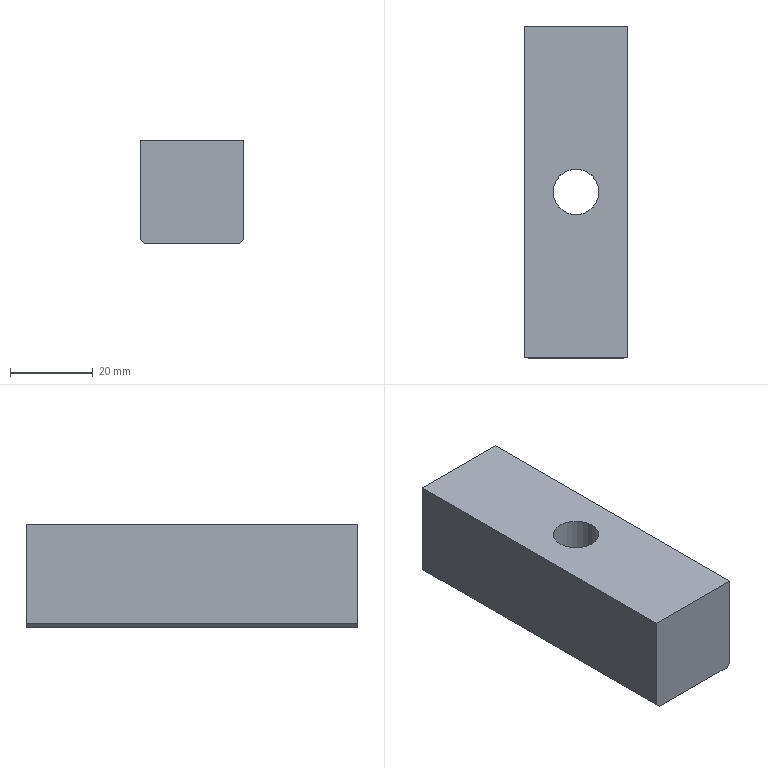Part | NX | features solid 2 | 1 solid | 11 faces | box 25 x 80 x 25 mm | volume 45631 mm3 | plane 9 | cylinder 2 | commonest cylinder face diameters 11 x1 18 x1
STEP:
#1=CARTESIAN_POINT('',(-5.5,1000.,-40.));
#2=VERTEX_POINT('',#1);
#3=CARTESIAN_POINT('',(0.,1000.,-40.));
#4=DIRECTION('',(0.,0.,-1.));
#5=DIRECTION('',(-1.,0.,0.));
#6=AXIS2_PLACEMENT_3D('',#3,#4,#5);
#7=CIRCLE('',#6,5.5);
#8=EDGE_CURVE('',#2,#2,#7,.T.);
#9=ORIENTED_EDGE('',*,*,#8,.T.);
#10=EDGE_LOOP('',(#9));
#11=FACE_BOUND('',#10,.T.);
#12=CARTESIAN_POINT('',(12.5,960.,-40.));
#13=VERTEX_POINT('',#12);
#14=CARTESIAN_POINT('',(-12.5,960.,-40.));
#15=VERTEX_POINT('',#14);
#16=CARTESIAN_POINT('',(0.,960.,-40.));
#17=DIRECTION('',(-1.,0.,0.));
#18=VECTOR('',#17,1000.);
#19=LINE('',#16,#18);
#20=EDGE_CURVE('',#13,#15,#19,.T.);
#21=ORIENTED_EDGE('',*,*,#20,.F.);
#22=CARTESIAN_POINT('',(12.5,1040.,-40.));
#23=VERTEX_POINT('',#22);
#24=CARTESIAN_POINT('',(12.5,1000.,-40.));
#25=DIRECTION('',(0.,-1.,0.));
#26=VECTOR('',#25,1000.);
#27=LINE('',#24,#26);
#28=EDGE_CURVE('',#23,#13,#27,.T.);
#29=ORIENTED_EDGE('',*,*,#28,.F.);
#30=CARTESIAN_POINT('',(-12.5,1040.,-40.));
#31=VERTEX_POINT('',#30);
#32=CARTESIAN_POINT('',(0.,1040.,-40.));
#33=DIRECTION('',(1.,0.,0.));
#34=VECTOR('',#33,1000.);
#35=LINE('',#32,#34);
#36=EDGE_CURVE('',#31,#23,#35,.T.);
#37=ORIENTED_EDGE('',*,*,#36,.F.);
#38=CARTESIAN_POINT('',(-12.5,1000.,-40.));
#39=DIRECTION('',(0.,1.,0.));
#40=VECTOR('',#39,1000.);
#41=LINE('',#38,#40);
#42=EDGE_CURVE('',#15,#31,#41,.T.);
#43=ORIENTED_EDGE('',*,*,#42,.F.);
#44=EDGE_LOOP('',(#21,#29,#37,#43));
#45=FACE_BOUND('',#44,.T.);
#46=CARTESIAN_POINT('',(0.,1000.,-40.));
#47=DIRECTION('',(0.,0.,1.));
#48=DIRECTION('',(1.,0.,0.));
#49=AXIS2_PLACEMENT_3D('',#46,#47,#48);
#50=PLANE('',#49);
#51=ADVANCED_FACE('',(#11,#45),#50,.T.);
#52=CARTESIAN_POINT('',(-11.5,960.,-65.));
#53=VERTEX_POINT('',#52);
#54=CARTESIAN_POINT('',(11.5,960.,-65.));
#55=VERTEX_POINT('',#54);
#56=CARTESIAN_POINT('',(0.,960.,-65.));
#57=DIRECTION('',(1.,0.,0.));
#58=VECTOR('',#57,1000.);
#59=LINE('',#56,#58);
#60=EDGE_CURVE('',#53,#55,#59,.T.);
#61=ORIENTED_EDGE('',*,*,#60,.T.);
#62=CARTESIAN_POINT('',(12.5,960.,-64.));
#63=VERTEX_POINT('',#62);
#64=CARTESIAN_POINT('',(5.75,960.,-70.75));
#65=DIRECTION('',(-0.7071,0.,-0.7071));
#66=VECTOR('',#65,1000.);
#67=LINE('',#64,#66);
#68=EDGE_CURVE('',#55,#63,#67,.F.);
#69=ORIENTED_EDGE('',*,*,#68,.T.);
#70=CARTESIAN_POINT('',(12.5,960.,-65.));
#71=DIRECTION('',(0.,0.,1.));
#72=VECTOR('',#71,1000.);
#73=LINE('',#70,#72);
#74=EDGE_CURVE('',#63,#13,#73,.T.);
#75=ORIENTED_EDGE('',*,*,#74,.T.);
#76=ORIENTED_EDGE('',*,*,#20,.T.);
#77=CARTESIAN_POINT('',(-12.5,960.,-64.));
#78=VERTEX_POINT('',#77);
#79=CARTESIAN_POINT('',(-12.5,960.,-65.));
#80=DIRECTION('',(0.,0.,1.));
#81=VECTOR('',#80,1000.);
#82=LINE('',#79,#81);
#83=EDGE_CURVE('',#78,#15,#82,.T.);
#84=ORIENTED_EDGE('',*,*,#83,.F.);
#85=CARTESIAN_POINT('',(-5.75,960.,-70.75));
#86=DIRECTION('',(-0.7071,0.,0.7071));
#87=VECTOR('',#86,1000.);
#88=LINE('',#85,#87);
#89=EDGE_CURVE('',#78,#53,#88,.F.);
#90=ORIENTED_EDGE('',*,*,#89,.T.);
#91=EDGE_LOOP('',(#61,#69,#75,#76,#84,#90));
#92=FACE_BOUND('',#91,.T.);
#93=CARTESIAN_POINT('',(0.,960.,-65.));
#94=DIRECTION('',(0.,-1.,0.));
#95=DIRECTION('',(0.,0.,-1.));
#96=AXIS2_PLACEMENT_3D('',#93,#94,#95);
#97=PLANE('',#96);
#98=ADVANCED_FACE('',(#92),#97,.T.);
#99=CARTESIAN_POINT('',(-12.5,1040.,-64.));
#100=VERTEX_POINT('',#99);
#101=CARTESIAN_POINT('',(-12.5,1040.,-65.));
#102=DIRECTION('',(0.,0.,1.));
#103=VECTOR('',#102,1000.);
#104=LINE('',#101,#103);
#105=EDGE_CURVE('',#100,#31,#104,.T.);
#106=ORIENTED_EDGE('',*,*,#105,.F.);
#107=CARTESIAN_POINT('',(-12.5,1000.,-64.));
#108=DIRECTION('',(0.,-1.,0.));
#109=VECTOR('',#108,1000.);
#110=LINE('',#107,#109);
#111=EDGE_CURVE('',#100,#78,#110,.T.);
#112=ORIENTED_EDGE('',*,*,#111,.T.);
#113=ORIENTED_EDGE('',*,*,#83,.T.);
#114=ORIENTED_EDGE('',*,*,#42,.T.);
#115=EDGE_LOOP('',(#106,#112,#113,#114));
#116=FACE_BOUND('',#115,.T.);
#117=CARTESIAN_POINT('',(-12.5,1000.,-65.));
#118=DIRECTION('',(-1.,0.,0.));
#119=DIRECTION('',(0.,0.,1.));
#120=AXIS2_PLACEMENT_3D('',#117,#118,#119);
#121=PLANE('',#120);
#122=ADVANCED_FACE('',(#116),#121,.T.);
#123=CARTESIAN_POINT('',(12.5,1040.,-64.));
#124=VERTEX_POINT('',#123);
#125=CARTESIAN_POINT('',(12.5,1040.,-65.));
#126=DIRECTION('',(0.,0.,1.));
#127=VECTOR('',#126,1000.);
#128=LINE('',#125,#127);
#129=EDGE_CURVE('',#124,#23,#128,.T.);
#130=ORIENTED_EDGE('',*,*,#129,.F.);
#131=CARTESIAN_POINT('',(11.5,1040.,-65.));
#132=VERTEX_POINT('',#131);
#133=CARTESIAN_POINT('',(5.75,1040.,-70.75));
#134=DIRECTION('',(0.7071,0.,0.7071));
#135=VECTOR('',#134,1000.);
#136=LINE('',#133,#135);
#137=EDGE_CURVE('',#124,#132,#136,.F.);
#138=ORIENTED_EDGE('',*,*,#137,.T.);
#139=CARTESIAN_POINT('',(-11.5,1040.,-65.));
#140=VERTEX_POINT('',#139);
#141=CARTESIAN_POINT('',(0.,1040.,-65.));
#142=DIRECTION('',(-1.,0.,0.));
#143=VECTOR('',#142,1000.);
#144=LINE('',#141,#143);
#145=EDGE_CURVE('',#132,#140,#144,.T.);
#146=ORIENTED_EDGE('',*,*,#145,.T.);
#147=CARTESIAN_POINT('',(-5.75,1040.,-70.75));
#148=DIRECTION('',(0.7071,0.,-0.7071));
#149=VECTOR('',#148,1000.);
#150=LINE('',#147,#149);
#151=EDGE_CURVE('',#140,#100,#150,.F.);
#152=ORIENTED_EDGE('',*,*,#151,.T.);
#153=ORIENTED_EDGE('',*,*,#105,.T.);
#154=ORIENTED_EDGE('',*,*,#36,.T.);
#155=EDGE_LOOP('',(#130,#138,#146,#152,#153,#154));
#156=FACE_BOUND('',#155,.T.);
#157=CARTESIAN_POINT('',(0.,1040.,-65.));
#158=DIRECTION('',(0.,1.,0.));
#159=DIRECTION('',(0.,0.,1.));
#160=AXIS2_PLACEMENT_3D('',#157,#158,#159);
#161=PLANE('',#160);
#162=ADVANCED_FACE('',(#156),#161,.T.);
#163=CARTESIAN_POINT('',(9.,1000.,-65.));
#164=VERTEX_POINT('',#163);
#165=CARTESIAN_POINT('',(0.,1000.,-65.));
#166=DIRECTION('',(0.,0.,1.));
#167=DIRECTION('',(1.,0.,0.));
#168=AXIS2_PLACEMENT_3D('',#165,#166,#167);
#169=CIRCLE('',#168,9.);
#170=EDGE_CURVE('',#164,#164,#169,.T.);
#171=ORIENTED_EDGE('',*,*,#170,.T.);
#172=EDGE_LOOP('',(#171));
#173=FACE_BOUND('',#172,.T.);
#174=ORIENTED_EDGE('',*,*,#145,.F.);
#175=CARTESIAN_POINT('',(11.5,1000.,-65.));
#176=DIRECTION('',(0.,-1.,0.));
#177=VECTOR('',#176,1000.);
#178=LINE('',#175,#177);
#179=EDGE_CURVE('',#132,#55,#178,.T.);
#180=ORIENTED_EDGE('',*,*,#179,.T.);
#181=ORIENTED_EDGE('',*,*,#60,.F.);
#182=CARTESIAN_POINT('',(-11.5,1000.,-65.));
#183=DIRECTION('',(0.,1.,0.));
#184=VECTOR('',#183,1000.);
#185=LINE('',#182,#184);
#186=EDGE_CURVE('',#53,#140,#185,.T.);
#187=ORIENTED_EDGE('',*,*,#186,.T.);
#188=EDGE_LOOP('',(#174,#180,#181,#187));
#189=FACE_BOUND('',#188,.T.);
#190=CARTESIAN_POINT('',(0.,1000.,-65.));
#191=DIRECTION('',(0.,0.,-1.));
#192=DIRECTION('',(-1.,0.,0.));
#193=AXIS2_PLACEMENT_3D('',#190,#191,#192);
#194=PLANE('',#193);
#195=ADVANCED_FACE('',(#173,#189),#194,.T.);
#196=ORIENTED_EDGE('',*,*,#74,.F.);
#197=CARTESIAN_POINT('',(12.5,1000.,-64.));
#198=DIRECTION('',(0.,1.,0.));
#199=VECTOR('',#198,1000.);
#200=LINE('',#197,#199);
#201=EDGE_CURVE('',#63,#124,#200,.T.);
#202=ORIENTED_EDGE('',*,*,#201,.T.);
#203=ORIENTED_EDGE('',*,*,#129,.T.);
#204=ORIENTED_EDGE('',*,*,#28,.T.);
#205=EDGE_LOOP('',(#196,#202,#203,#204));
#206=FACE_BOUND('',#205,.T.);
#207=CARTESIAN_POINT('',(12.5,1000.,-65.));
#208=DIRECTION('',(1.,0.,0.));
#209=DIRECTION('',(0.,0.,-1.));
#210=AXIS2_PLACEMENT_3D('',#207,#208,#209);
#211=PLANE('',#210);
#212=ADVANCED_FACE('',(#206),#211,.T.);
#213=CARTESIAN_POINT('',(5.5,1000.,-53.));
#214=VERTEX_POINT('',#213);
#215=CARTESIAN_POINT('',(0.,1000.,-53.));
#216=DIRECTION('',(0.,0.,1.));
#217=DIRECTION('',(1.,0.,0.));
#218=AXIS2_PLACEMENT_3D('',#215,#216,#217);
#219=CIRCLE('',#218,5.5);
#220=EDGE_CURVE('',#214,#214,#219,.F.);
#221=ORIENTED_EDGE('',*,*,#220,.T.);
#222=EDGE_LOOP('',(#221));
#223=FACE_BOUND('',#222,.T.);
#224=ORIENTED_EDGE('',*,*,#8,.F.);
#225=EDGE_LOOP('',(#224));
#226=FACE_BOUND('',#225,.T.);
#227=CARTESIAN_POINT('',(0.,1000.,-40.));
#228=DIRECTION('',(0.,0.,-1.));
#229=DIRECTION('',(-1.,0.,0.));
#230=AXIS2_PLACEMENT_3D('',#227,#228,#229);
#231=CYLINDRICAL_SURFACE('',#230,5.5);
#232=ADVANCED_FACE('',(#223,#226),#231,.F.);
#233=CARTESIAN_POINT('',(-9.,1000.,-53.));
#234=VERTEX_POINT('',#233);
#235=CARTESIAN_POINT('',(0.,1000.,-53.));
#236=DIRECTION('',(0.,0.,-1.));
#237=DIRECTION('',(-1.,0.,0.));
#238=AXIS2_PLACEMENT_3D('',#235,#236,#237);
#239=CIRCLE('',#238,9.);
#240=EDGE_CURVE('',#234,#234,#239,.T.);
#241=ORIENTED_EDGE('',*,*,#240,.T.);
#242=EDGE_LOOP('',(#241));
#243=FACE_BOUND('',#242,.T.);
#244=ORIENTED_EDGE('',*,*,#220,.F.);
#245=EDGE_LOOP('',(#244));
#246=FACE_BOUND('',#245,.T.);
#247=CARTESIAN_POINT('',(0.,1000.,-53.));
#248=DIRECTION('',(0.,0.,1.));
#249=DIRECTION('',(1.,0.,0.));
#250=AXIS2_PLACEMENT_3D('',#247,#248,#249);
#251=PLANE('',#250);
#252=ADVANCED_FACE('',(#243,#246),#251,.F.);
#253=ORIENTED_EDGE('',*,*,#170,.F.);
#254=EDGE_LOOP('',(#253));
#255=FACE_BOUND('',#254,.T.);
#256=ORIENTED_EDGE('',*,*,#240,.F.);
#257=EDGE_LOOP('',(#256));
#258=FACE_BOUND('',#257,.T.);
#259=CARTESIAN_POINT('',(0.,1000.,-53.));
#260=DIRECTION('',(0.,0.,-1.));
#261=DIRECTION('',(-1.,0.,0.));
#262=AXIS2_PLACEMENT_3D('',#259,#260,#261);
#263=CYLINDRICAL_SURFACE('',#262,9.);
#264=ADVANCED_FACE('',(#255,#258),#263,.F.);
#265=ORIENTED_EDGE('',*,*,#68,.F.);
#266=ORIENTED_EDGE('',*,*,#179,.F.);
#267=ORIENTED_EDGE('',*,*,#137,.F.);
#268=ORIENTED_EDGE('',*,*,#201,.F.);
#269=EDGE_LOOP('',(#265,#266,#267,#268));
#270=FACE_BOUND('',#269,.T.);
#271=CARTESIAN_POINT('',(12.5,1000.,-64.));
#272=DIRECTION('',(-0.7071,0.,0.7071));
#273=DIRECTION('',(0.7071,0.,0.7071));
#274=AXIS2_PLACEMENT_3D('',#271,#272,#273);
#275=PLANE('',#274);
#276=ADVANCED_FACE('',(#270),#275,.F.);
#277=ORIENTED_EDGE('',*,*,#151,.F.);
#278=ORIENTED_EDGE('',*,*,#186,.F.);
#279=ORIENTED_EDGE('',*,*,#89,.F.);
#280=ORIENTED_EDGE('',*,*,#111,.F.);
#281=EDGE_LOOP('',(#277,#278,#279,#280));
#282=FACE_BOUND('',#281,.T.);
#283=CARTESIAN_POINT('',(-12.5,1000.,-64.));
#284=DIRECTION('',(0.7071,0.,0.7071));
#285=DIRECTION('',(0.7071,0.,-0.7071));
#286=AXIS2_PLACEMENT_3D('',#283,#284,#285);
#287=PLANE('',#286);
#288=ADVANCED_FACE('',(#282),#287,.F.);
#289=CLOSED_SHELL('',(#51,#98,#122,#162,#195,#212,#232,#252,#264,#276,#288));
#290=MANIFOLD_SOLID_BREP('',#289);
#291=(LENGTH_UNIT()NAMED_UNIT(*)SI_UNIT(.MILLI.,.METRE.));
#292=UNCERTAINTY_MEASURE_WITH_UNIT(LENGTH_MEASURE(0.00001),#291,'','');
#293=(NAMED_UNIT(*)PLANE_ANGLE_UNIT()SI_UNIT($,.RADIAN.));
#294=(NAMED_UNIT(*)SI_UNIT($,.STERADIAN.)SOLID_ANGLE_UNIT());
#295=(GEOMETRIC_REPRESENTATION_CONTEXT(3)GLOBAL_UNCERTAINTY_ASSIGNED_CONTEXT((#292))GLOBAL_UNIT_ASSIGNED_CONTEXT((#291,#293,#294))REPRESENTATION_CONTEXT('',''));
#296=ADVANCED_BREP_SHAPE_REPRESENTATION('',(#290),#295);